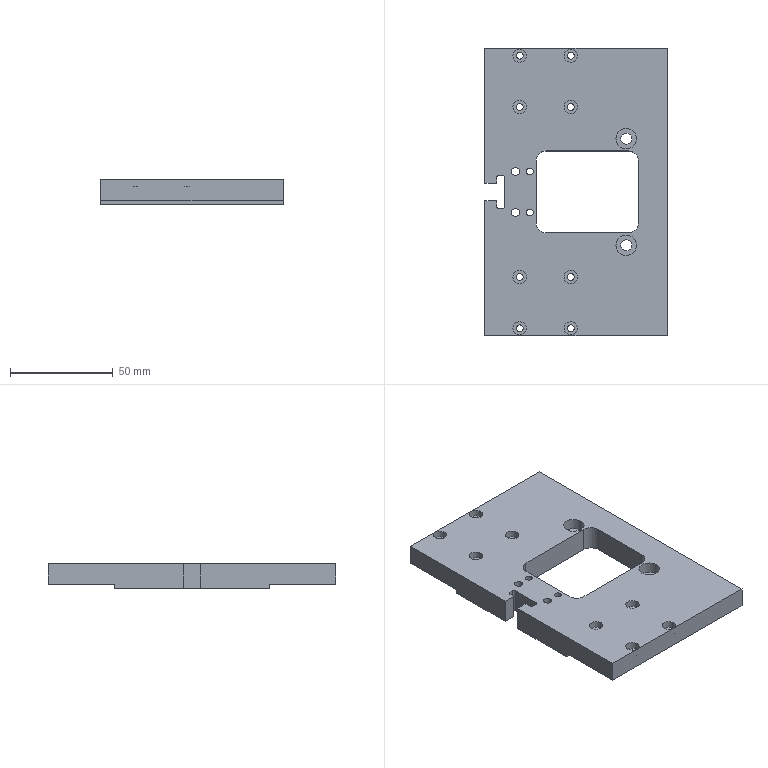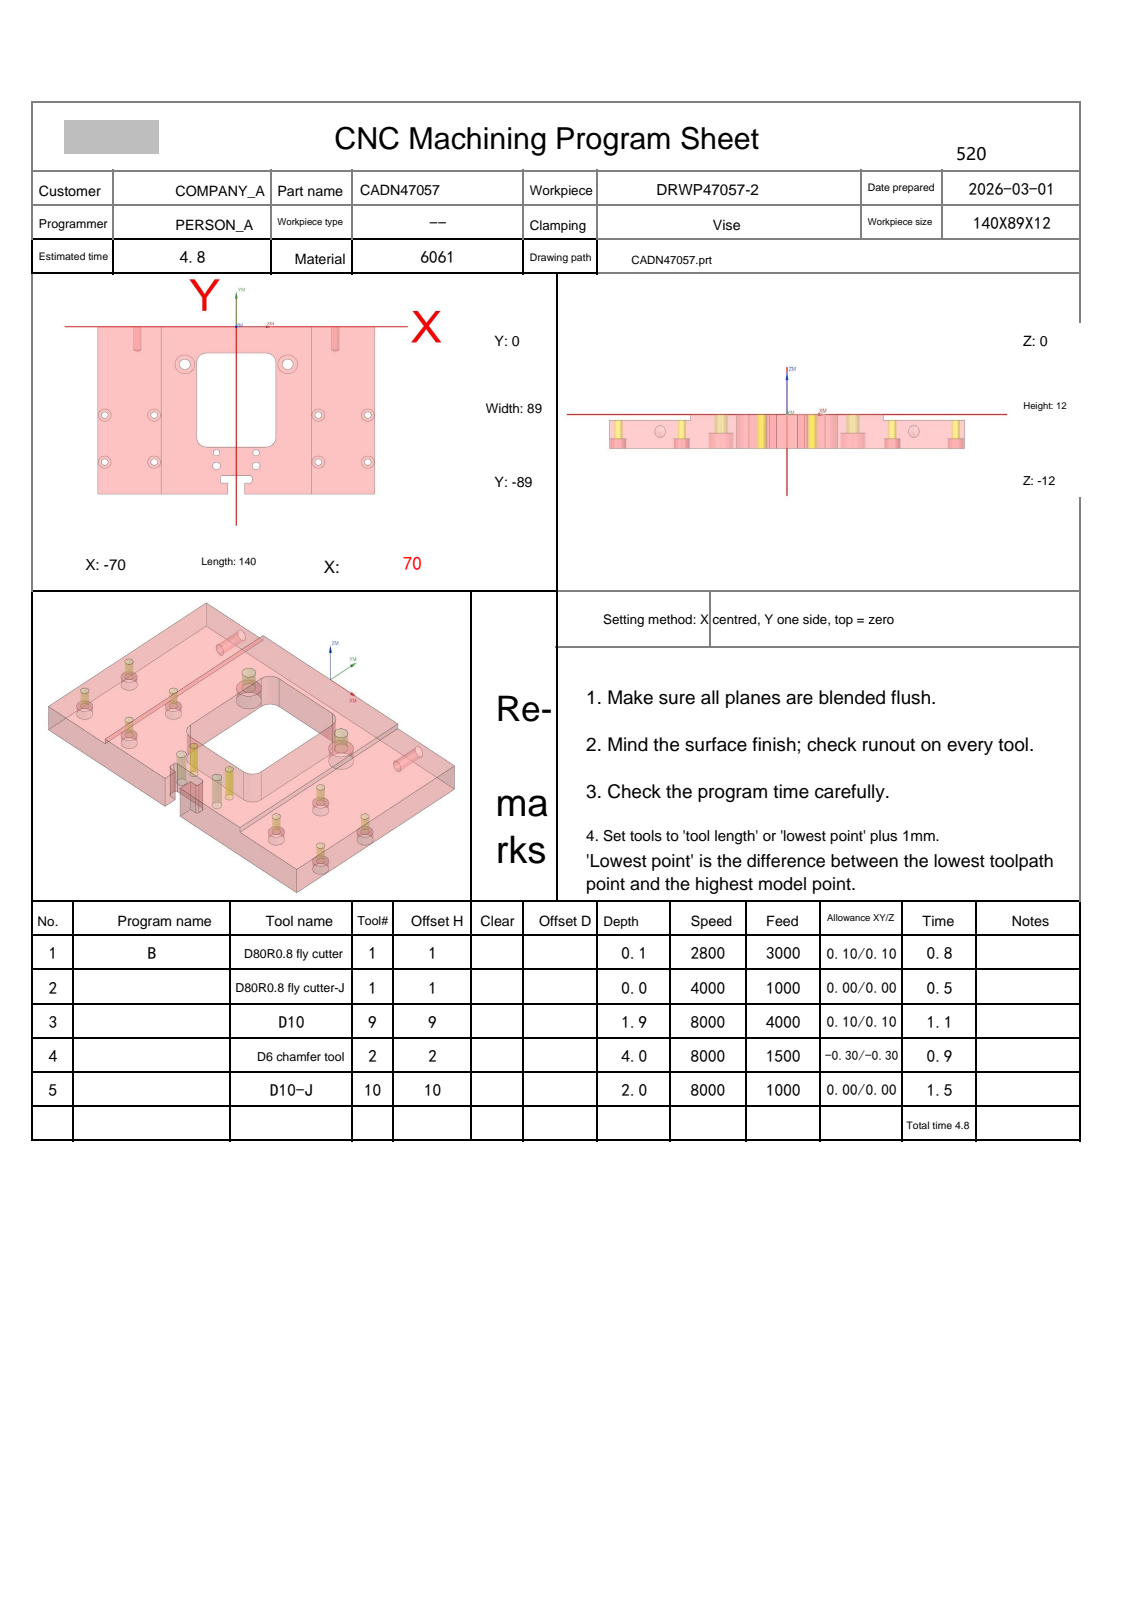NC program | NX | posted by the shop | part box 89 x 140 x 12 mm
Whole program:
%
O0001
(Machine time: 5.83 MIN)
(===Total Tool:4===)
(T1=D80R0.8 fly cutter D=80.  R=0.8  D-  H01 Z=0.    )
(T9=D10     D=10.  R=0.   D-  H09 Z=-1.9  )
(T2=D6 chamfer tool   D=6.   R=0.   D-  H02 Z=-4.   )
(T10=D10-J  D=10.  R=0.   D10 H10 Z=-2.   )
G80 G90 G17 G49 G40
G91 G28 Z0
M01
N1 T01 M06
(D80R0.8 fly cutter  D=80. R=0.8 H=01 ce=0.10 di=0.10)
G00 G90 G54 X-122.097 Y-23.903 M03 S2800
G43 H01 Z50.
M08
Z4.02
G01 Z2.02 F3000.
X-110.097
X102.897
G02 X110.097 Y-31.103 I0.0 J-7.2
G01 Y-49.737
G02 X102.097 Y-57.737 I-8. J0.0
G01 X-110.097
X-122.097
Z4.02
G00 Y-23.903
Z3.54
G01 Z1.54
X-110.097
X102.897
G02 X110.097 Y-31.103 I0.0 J-7.2
G01 Y-49.737
G02 X102.097 Y-57.737 I-8. J0.0
G01 X-110.097
X-122.097
Z3.54
G00 Y-23.903
Z3.06
G01 Z1.06
X-110.097
X102.897
G02 X110.097 Y-31.103 I0.0 J-7.2
G01 Y-49.737
G02 X102.097 Y-57.737 I-8. J0.0
G01 X-110.097
X-122.097
Z3.06
G00 Y-23.903
Z2.58
G01 Z.58
X-110.097
X102.897
G02 X110.097 Y-31.103 I0.0 J-7.2
G01 Y-49.737
G02 X102.097 Y-57.737 I-8. J0.0
G01 X-110.097
X-122.097
Z2.58
G00 Y-23.903
Z2.1
G01 Z.1
X-110.097
X102.897
G02 X110.097 Y-31.103 I0.0 J-7.2
G01 Y-49.737
G02 X102.097 Y-57.737 I-8. J0.0
G01 X-110.097
X-122.097
Z2.1
G00 Z50.
G91 G28 Z0.0
M05
M09
G91 G28 Z0.0
M01
N2 T01 M06
(D80R0.8 fly cutter-J  D=80. R=0.8 H=01 ce=0.00 di=0.00)
G00 G90 G54 X-121.999 Y-24.001 M03 S4000
G43 H01 Z50.
M08
Z2.
G01 Z0.0 F1000.
X-109.999
X102.799
G02 X109.999 Y-31.201 I0.0 J-7.2
G01 Y-49.639
G02 X101.999 Y-57.639 I-8. J0.0
G01 X-109.999
X-121.999
Z2.
G00 Z50.
G91 G28 Z0.0
M05
M09
G91 G28 Z0.0
M01
N3 T09 M06
(D10  D=10. R=0. H=09 ce=0.10 di=0.10)
G00 G90 G54 X-73.1 Y-97. M03 S8000
G43 H09 Z12.5
M08
Z1.025
G01 Z-.475 F4000.
Y-93.9
Y3.901
G02 X-72.101 Y4.9 I1. J-.001
G01 X-70.
X-66.599
G02 X-65.6 Y3.901 I-.001 J-1.
G01 Y-92.901
G03 X-64.601 Y-93.9 I1. J.001
G01 X-59.099
G03 X-58.1 Y-92.901 I-.001 J1.
G01 Y3.901
G02 X-57.101 Y4.9 I1. J-.001
G01 X-51.599
G02 X-50.6 Y3.901 I-.001 J-1.
G01 Y-93.044
G03 X-49.755 Y-94.032 I1. J.001
G01 X-44.254 Y-94.888
X-44.1 Y-94.9
G03 X-43.1 Y-93.9 I0.0 J1.
G01 Y4.9
Y8.1
Z1.025
G00 X-73.1 Y-97.
Z.55
G01 Z-.95
Y-93.9
Y3.901
G02 X-72.101 Y4.9 I1. J-.001
G01 X-70.
X-66.599
G02 X-65.6 Y3.901 I-.001 J-1.
G01 Y-92.901
G03 X-64.601 Y-93.9 I1. J.001
G01 X-59.099
G03 X-58.1 Y-92.901 I-.001 J1.
G01 Y3.901
G02 X-57.101 Y4.9 I1. J-.001
G01 X-51.599
G02 X-50.6 Y3.901 I-.001 J-1.
G01 Y-93.044
G03 X-49.755 Y-94.032 I1. J.001
G01 X-44.254 Y-94.888
X-44.1 Y-94.9
G03 X-43.1 Y-93.9 I0.0 J1.
G01 Y4.9
Y8.1
Z.55
G00 X-73.1 Y-97.
Z.075
G01 Z-1.425
Y-93.9
Y3.901
G02 X-72.101 Y4.9 I1. J-.001
G01 X-70.
X-66.599
G02 X-65.6 Y3.901 I-.001 J-1.
G01 Y-92.901
G03 X-64.601 Y-93.9 I1. J.001
G01 X-59.099
G03 X-58.1 Y-92.901 I-.001 J1.
G01 Y3.901
G02 X-57.101 Y4.9 I1. J-.001
G01 X-51.599
G02 X-50.6 Y3.901 I-.001 J-1.
G01 Y-93.044
G03 X-49.755 Y-94.032 I1. J.001
G01 X-44.254 Y-94.888
X-44.1 Y-94.9
G03 X-43.1 Y-93.9 I0.0 J1.
G01 Y4.9
Y8.1
Z.075
G00 X-73.1 Y-97.
Z-.4
G01 Z-1.9
Y-93.9
Y3.901
G02 X-72.101 Y4.9 I1. J-.001
G01 X-70.
X-66.599
G02 X-65.6 Y3.901 I-.001 J-1.
G01 Y-92.901
G03 X-64.601 Y-93.9 I1. J.001
G01 X-59.099
G03 X-58.1 Y-92.901 I-.001 J1.
G01 Y3.901
G02 X-57.101 Y4.9 I1. J-.001
G01 X-51.599
G02 X-50.6 Y3.901 I-.001 J-1.
G01 Y-93.044
G03 X-49.755 Y-94.032 I1. J.001
G01 X-44.254 Y-94.888
X-44.1 Y-94.9
G03 X-43.1 Y-93.9 I0.0 J1.
G01 Y4.9
Y8.1
Z-.4
G00 Z3.
X73.1 Y8.
Z1.025
G01 Z-.475
Y4.9
Y-92.901
G02 X72.101 Y-93.9 I-1. J.001
G01 X66.599
G02 X65.6 Y-92.901 I.001 J1.
G01 Y3.901
G03 X64.601 Y4.9 I-1. J-.001
G01 X59.099
G03 X58.1 Y3.901 I.001 J-1.
G01 Y-92.901
G02 X57.101 Y-93.9 I-1. J.001
G01 X51.599
G02 X50.6 Y-92.901 I.001 J1.
G01 Y4.044
G03 X49.755 Y5.032 I-1. J-.001
G01 X44.254 Y5.888
X44.1 Y5.9
G03 X43.1 Y4.9 I0.0 J-1.
G01 Y-93.9
Y-97.1
Z1.025
G00 X73.1 Y8.
Z.55
G01 Z-.95
Y4.9
Y-92.901
G02 X72.101 Y-93.9 I-1. J.001
G01 X66.599
G02 X65.6 Y-92.901 I.001 J1.
G01 Y3.901
G03 X64.601 Y4.9 I-1. J-.001
G01 X59.099
G03 X58.1 Y3.901 I.001 J-1.
G01 Y-92.901
G02 X57.101 Y-93.9 I-1. J.001
G01 X51.599
G02 X50.6 Y-92.901 I.001 J1.
G01 Y4.044
G03 X49.755 Y5.032 I-1. J-.001
G01 X44.254 Y5.888
X44.1 Y5.9
G03 X43.1 Y4.9 I0.0 J-1.
G01 Y-93.9
Y-97.1
Z.55
G00 X73.1 Y8.
Z.075
G01 Z-1.425
Y4.9
Y-92.901
G02 X72.101 Y-93.9 I-1. J.001
G01 X66.599
G02 X65.6 Y-92.901 I.001 J1.
G01 Y3.901
G03 X64.601 Y4.9 I-1. J-.001
G01 X59.099
G03 X58.1 Y3.901 I.001 J-1.
G01 Y-92.901
G02 X57.101 Y-93.9 I-1. J.001
G01 X51.599
G02 X50.6 Y-92.901 I.001 J1.
G01 Y4.044
G03 X49.755 Y5.032 I-1. J-.001
G01 X44.254 Y5.888
X44.1 Y5.9
G03 X43.1 Y4.9 I0.0 J-1.
G01 Y-93.9
Y-97.1
Z.075
G00 X73.1 Y8.
Z-.4
G01 Z-1.9
Y4.9
Y-92.901
G02 X72.101 Y-93.9 I-1. J.001
G01 X66.599
G02 X65.6 Y-92.901 I.001 J1.
G01 Y3.901
G03 X64.601 Y4.9 I-1. J-.001
G01 X59.099
G03 X58.1 Y3.901 I.001 J-1.
G01 Y-92.901
G02 X57.101 Y-93.9 I-1. J.001
G01 X51.599
G02 X50.6 Y-92.901 I.001 J1.
G01 Y4.044
G03 X49.755 Y5.032 I-1. J-.001
G01 X44.254 Y5.888
X44.1 Y5.9
G03 X43.1 Y4.9 I0.0 J-1.
G01 Y-93.9
Y-97.1
Z-.4
G00 Z12.5
G91 G28 Z0.0
M05
M09
G91 G28 Z0.0
M01
N4 T02 M06
(D6 chamfer tool  D=6. R=0. H=02 ce=0.00 di=0.10)
G00 G90 G54 X-10. Y-67. M03 S8000
G43 H02 Z50.
M08
G98 G81 X-10. Y-67. Z-2.2 R3. F1000.
X10.
G80
G00 Z50.
G00 G90 X-66.5 Y-72. M03 S8000
Z50.
G98 G81 X-66.5 Y-72. Z-4. R1. F1000.
Y-47.
X-41.5
Y-72.
X41.5
Y-47.
X66.5
Y-72.
G80
G00 Z50.
G00 G90 X10. Y-74. M03 S8000
Z50.
G98 G81 X10. Y-74. Z-2.3 R3. F1000.
X-10.
G80
G00 Z50.
G00 G90 X25.353 Y-20.065 M03 S8000
Z50.
Z-.9
G01 Z-1.4 F1200.
X24.5 Y-20.15
G03 X26. Y-21.65 I1.5 J0.0
X27.65 Y-20. I0.0 J1.65
X26. Y-18.35 I-1.65 J0.0
X24.35 Y-20. I0.0 J-1.65
X26. Y-21.65 I1.65 J0.0
X27.5 Y-20.15 I0.0 J1.5
G01 X26.647 Y-20.065
Z-.9
G00 Z50.
X-26.647
Z-.9
G01 Z-1.4
X-27.5 Y-20.15
G03 X-26. Y-21.65 I1.5 J0.0
X-24.35 Y-20. I0.0 J1.65
X-26. Y-18.35 I-1.65 J0.0
X-27.65 Y-20. I0.0 J-1.65
X-26. Y-21.65 I1.65 J0.0
X-24.5 Y-20.15 I0.0 J1.5
G01 X-25.353 Y-20.065
Z-.9
G00 Z50.
G00 G90 X39.227 Y-44.114 M03 S6500
Z50.
Z.172
G01 Z-1.2 F1500.
G03 X39.027 Y-44.4 I1.532 J-1.286
G01 X38.997 Y-44.446
X39. Y-44.5
Y-89.
G02 X38. Y-90. I-1. J0.0
G01 X4.25
G02 X3.25 Y-89. I0.0 J1.
G01 Y-83.2
G02 X4.25 Y-82.2 I1. J0.0
G01 X7.
Y-80.2
X-7.
Y-82.2
X-4.25
G02 X-3.25 Y-83.2 I0.0 J-1.
G01 Y-89.
G02 X-4.25 Y-90. I-1. J0.0
G01 X-38.
G02 X-39. Y-89. I0.0 J1.
G01 Y0.0
G02 X-38. Y1. I1. J0.0
G01 X38.
G02 X39. Y0.0 I0.0 J-1.
G01 Y-44.5
X38.997 Y-44.554
X39.027 Y-44.6
G03 X39.227 Y-44.886 I1.732 J1.
G01 Z.172
G00 Z10.
X-10.412 Y-74.826
Z.33
G01 Z-1.2
G03 X-10.103 Y-74.986 I1.075 J1.687
G01 X-10.054 Y-75.01
X-10. Y-75.
G03 X-9. Y-74. I0.0 J1.
X-10. Y-73. I-1. J0.0
X-11. Y-74. I0.0 J-1.
X-10. Y-75. I1. J0.0
G01 X-9.946 Y-75.01
X-9.897 Y-74.986
G03 X-9.588 Y-74.826 I-.765 J1.848
G01 Z.33
G00 Z2.55
X-10.419 Y-67.494
Z.405
G01 Z-1.2
G03 X-10.103 Y-67.641 I1. J1.732
G01 X-10.053 Y-67.662
X-10. Y-67.65
G03 X-9.35 Y-67. I0.0 J.65
X-10. Y-66.35 I-.65 J0.0
X-10.65 Y-67. I0.0 J-.65
X-10. Y-67.65 I.65 J0.0
G01 X-9.947 Y-67.662
X-9.897 Y-67.641
G03 X-9.581 Y-67.494 I-.684 J1.879
G01 Z.405
G00 Z10.
X9.588 Y-74.826
Z.33
G01 Z-1.2
G03 X9.897 Y-74.986 I1.075 J1.687
G01 X9.946 Y-75.01
X10. Y-75.
G03 X11. Y-74. I0.0 J1.
X10. Y-73. I-1. J0.0
X9. Y-74. I0.0 J-1.
X10. Y-75. I1. J0.0
G01 X10.054 Y-75.01
X10.103 Y-74.986
G03 X10.412 Y-74.826 I-.765 J1.848
G01 Z.33
G00 Z2.55
X9.581 Y-67.494
Z.405
G01 Z-1.2
G03 X9.897 Y-67.641 I1. J1.732
G01 X9.947 Y-67.662
X10. Y-67.65
G03 X10.65 Y-67. I0.0 J.65
X10. Y-66.35 I-.65 J0.0
X9.35 Y-67. I0.0 J-.65
X10. Y-67.65 I.65 J0.0
G01 X10.053 Y-67.662
X10.103 Y-67.641
G03 X10.419 Y-67.494 I-.684 J1.879
G01 Z.405
G00 Z10.
X18.773 Y-39.386
Z.172
G01 Z-1.2
G03 X18.973 Y-39.1 I-1.532 J1.286
G01 X19.003 Y-39.054
X19. Y-39.
Y-19.
G03 X15. Y-15. I-4. J0.0
G01 X-15.
G03 X-19. Y-19. I0.0 J-4.
G01 Y-59.
G03 X-15. Y-63. I4. J0.0
G01 X15.
G03 X19. Y-59. I0.0 J4.
G01 Y-39.
X19.003 Y-38.946
X18.973 Y-38.9
G03 X18.773 Y-38.614 I-1.732 J-1.
G01 Z.172
G00 Z10.
X-26.407 Y-21.565
Z.27
G01 Z-1.2
G03 X-26.102 Y-21.734 I1.118 J1.658
G01 X-26.054 Y-21.759
X-26. Y-21.75
G03 X-24.25 Y-20. I0.0 J1.75
X-26. Y-18.25 I-1.75 J0.0
X-27.75 Y-20. I0.0 J-1.75
X-26. Y-21.75 I1.75 J0.0
G01 X-25.946 Y-21.759
X-25.898 Y-21.734
G03 X-25.593 Y-21.565 I-.813 J1.827
G01 Z.27
G00 Z10.
X25.593
Z.27
G01 Z-1.2
G03 X25.898 Y-21.734 I1.118 J1.658
G01 X25.946 Y-21.759
X26. Y-21.75
G03 X27.75 Y-20. I0.0 J1.75
X26. Y-18.25 I-1.75 J0.0
X24.25 Y-20. I0.0 J-1.75
X26. Y-21.75 I1.75 J0.0
G01 X26.054 Y-21.759
X26.102 Y-21.734
G03 X26.407 Y-21.565 I-.813 J1.827
G01 Z.27
G00 Z10.
X40.978 Y1.068
Z-1.669
G01 Z-3.199
X41.064 Y1.008
X41.094 Y1.
X70.
G02 X71. Y0.0 I0.0 J-1.
G01 Y-89.
G02 X70. Y-90. I-1. J0.0
G01 X41.094
X41.064 Y-90.008
X40.978 Y-90.068
Z-1.669
G00 Z10.
X41.169 Y-72.516
Z-1.68
G01 Z-3.199
X41.195 Y-72.582
X41.244 Y-72.633
X41.252 Y-72.656
X41.277 Y-72.659
X41.319 Y-72.676
X41.5 Y-72.7
G03 X42.2 Y-72. I0.0 J.7
X41.5 Y-71.3 I-.7 J0.0
X41.294 Y-71.331 I0.0 J-.7
G01 X41.247 Y-71.354
X41.223 Y-71.374
X41.172 Y-71.465
Z-1.664
G00 Z10.
X66.088 Y-72.526
Z-1.624
G01 Z-3.199
G03 X66.397 Y-72.686 I1.075 J1.687
G01 X66.446 Y-72.71
X66.5 Y-72.7
G03 X67.2 Y-72. I0.0 J.7
X66.5 Y-71.3 I-.7 J0.0
X65.8 Y-72. I0.0 J-.7
X66.319 Y-72.676 I.7 J0.0
G01 X66.5 Y-72.7
X66.554 Y-72.71
X66.603 Y-72.686
G03 X66.912 Y-72.526 I-.765 J1.848
G01 Z-1.624
G00 Z10.
X66.088 Y-47.526
Z-1.624
G01 Z-3.199
G03 X66.397 Y-47.686 I1.075 J1.687
G01 X66.446 Y-47.71
X66.5 Y-47.7
G03 X67.2 Y-47. I0.0 J.7
X66.5 Y-46.3 I-.7 J0.0
X65.8 Y-47. I0.0 J-.7
X66.319 Y-47.676 I.7 J0.0
G01 X66.5 Y-47.7
X66.554 Y-47.71
X66.603 Y-47.686
G03 X66.912 Y-47.526 I-.765 J1.848
G01 Z-1.624
G00 Z10.
X41.169 Y-47.516
Z-1.68
G01 Z-3.199
X41.195 Y-47.582
X41.244 Y-47.633
X41.252 Y-47.656
X41.277 Y-47.659
X41.319 Y-47.676
X41.5 Y-47.7
G03 X42.2 Y-47. I0.0 J.7
X41.5 Y-46.3 I-.7 J0.0
X41.294 Y-46.331 I0.0 J-.7
G01 X41.247 Y-46.354
X41.223 Y-46.374
X41.172 Y-46.465
Z-1.664
G00 Z10.
X-40.978 Y-90.068
Z-1.669
G01 Z-3.199
X-41.064 Y-90.008
X-41.094 Y-90.
X-70.
G02 X-71. Y-89. I0.0 J1.
G01 Y0.0
G02 X-70. Y1. I1. J0.0
G01 X-41.094
X-41.064 Y1.008
X-40.978 Y1.068
Z-1.669
G00 Z10.
X-66.912 Y-72.526
Z-1.624
G01 Z-3.199
G03 X-66.603 Y-72.686 I1.075 J1.687
G01 X-66.554 Y-72.71
X-66.5 Y-72.7
G03 X-65.8 Y-72. I0.0 J.7
X-66.5 Y-71.3 I-.7 J0.0
X-67.2 Y-72. I0.0 J-.7
X-66.681 Y-72.676 I.7 J0.0
G01 X-66.5 Y-72.7
X-66.446 Y-72.71
X-66.397 Y-72.686
G03 X-66.088 Y-72.526 I-.765 J1.848
G01 Z-1.624
G00 Z10.
X-66.912 Y-47.526
Z-1.624
G01 Z-3.199
G03 X-66.603 Y-47.686 I1.075 J1.687
G01 X-66.554 Y-47.71
X-66.5 Y-47.7
G03 X-65.8 Y-47. I0.0 J.7
X-66.5 Y-46.3 I-.7 J0.0
X-67.2 Y-47. I0.0 J-.7
X-66.681 Y-47.676 I.7 J0.0
G01 X-66.5 Y-47.7
X-66.446 Y-47.71
X-66.397 Y-47.686
G03 X-66.088 Y-47.526 I-.765 J1.848
G01 Z-1.624
G00 Z10.
X-41.172 Y-46.465
Z-1.664
G01 Z-3.199
X-41.223 Y-46.374
X-41.247 Y-46.354
X-41.294 Y-46.331
G03 X-41.5 Y-46.3 I-.206 J-.669
X-42.2 Y-47. I0.0 J-.7
G01 X-42.182 Y-47.156
G03 X-41.506 Y-47.698 I.677 J.151
X-41.277 Y-47.659 I0.0 J.693
G01 X-41.252 Y-47.656
X-41.244 Y-47.633
X-41.195 Y-47.582
X-41.169 Y-47.516
Z-1.68
G00 Z10.
X-41.172 Y-71.465
Z-1.664
G01 Z-3.199
X-41.223 Y-71.374
X-41.247 Y-71.354
X-41.294 Y-71.331
G03 X-41.5 Y-71.3 I-.206 J-.669
X-42.2 Y-72. I0.0 J-.7
X-41.5 Y-72.7 I.7 J0.0
G01 X-41.319 Y-72.676
X-41.277 Y-72.659
X-41.252 Y-72.656
X-41.244 Y-72.633
X-41.195 Y-72.582
X-41.169 Y-72.516
Z-1.68
G00 Z50.
G91 G28 Z0.0
M05
M09
G91 G28 Z0.0
M01
N5 T10 M06
(D10-J  D=10. R=0. H=10 ce=0.40 di=0.00)
G00 G90 G54 X-77. Y-46.5 M03 S8000
G43 H10 Z12.5
M08
Z-.5
G01 Z-2. F1000.
X-73.
G03 X-71. Y-44.5 I0.0 J2.
G01 Y.003
G02 X-70. Y1. I1. J-.003
G01 X-44.397
G02 X-43.4 Y.003 I-.003 J-1.
G01 Y-89.003
G02 X-44.397 Y-90. I-1. J.003
G01 X-70.003
G02 X-71. Y-89.003 I.003 J1.
G01 Y-42.414
G02 X-70.708 Y-41.708 I1. J-.001
G01 X-66.293 Y-37.293
G03 X-66. Y-36.586 I-.707 J.707
G01 Y-4.997
G02 X-65.003 Y-4. I1. J-.003
G01 X-49.397
G02 X-48.4 Y-4.997 I-.003 J-1.
G01 Y-84.003
G02 X-49.397 Y-85. I-1. J.003
G01 X-65.003
G02 X-66. Y-84.003 I.003 J1.
G01 Y-42.414
G02 X-65.707 Y-41.707 I1. J-.001
G01 X-61.293 Y-37.293
G03 X-61. Y-36.586 I-.707 J.707
G01 Y-9.997
G02 X-60.003 Y-9. I1. J-.003
G01 X-54.397
G02 X-53.4 Y-9.997 I-.003 J-1.
G01 Y-79.003
G02 X-54.397 Y-80. I-1. J.003
G01 X-60.003
G02 X-61. Y-79.003 I.003 J1.
G01 Y-39.5
Y-38.5
G03 X-63. Y-36.5 I-2. J0.0
G01 Z-.5
G00 Z12.5
X77. Y-42.5
Z-.5
G01 Z-2.
X73.
G03 X71. Y-44.5 I0.0 J-2.
G01 Y-89.003
G02 X70.003 Y-90. I-1. J.003
G01 X44.397
G02 X43.4 Y-89.003 I.003 J1.
G01 Y.003
G02 X44.397 Y1. I1. J-.003
G01 X70.003
G02 X71. Y0.0 I-.003 J-1.
G01 Y-49.5
G02 X70.338 Y-50.441 I-1. J0.0
G01 X66.661 Y-51.762
G03 X66. Y-52.703 I.339 J-.941
G01 Y-84.003
G02 X65.003 Y-85. I-1. J.003
G01 X49.397
G02 X48.4 Y-84.003 I.003 J1.
G01 Y-4.997
G02 X49.397 Y-4. I1. J-.003
G01 X65.003
G02 X66. Y-4.997 I-.003 J-1.
G01 Y-46.586
G02 X65.708 Y-47.293 I-1. J.001
G01 X61.293 Y-51.707
G03 X61. Y-52.414 I.707 J-.707
G01 Y-79.003
G02 X60.003 Y-80. I-1. J.003
G01 X54.397
G02 X53.4 Y-79.003 I.003 J1.
G01 Y-9.997
G02 X54.397 Y-9. I1. J-.003
G01 X60.003
G02 X61. Y-9.997 I-.003 J-1.
G01 Y-49.5
Y-50.5
G03 X63. Y-52.5 I2. J0.0
G01 Z-.5
G00 Z12.5
G00 G90 X-45.199 Y-96. M03 S8000
Z12.5
Z-1.
G01 Z-2. F1000.
G41 D10
X-44.999
G03 X-43. Y-94. I-.001 J2.
G01 Y5.
G03 X-44.999 Y7. I-2. J0.0
G01 G40 X-45.199
Z-1.
G00 Z3.
X45.199
Z-1.
G01 Z-2.
G41 D10
X44.999
G03 X43. Y5. I.001 J-2.
G01 Y-94.
G03 X44.999 Y-96. I2. J0.0
G01 G40 X45.199
Z-1.
G00 Z12.5
M05
M09
G91 G28 Z0.0
G91 G28 Y0.0
M30
%